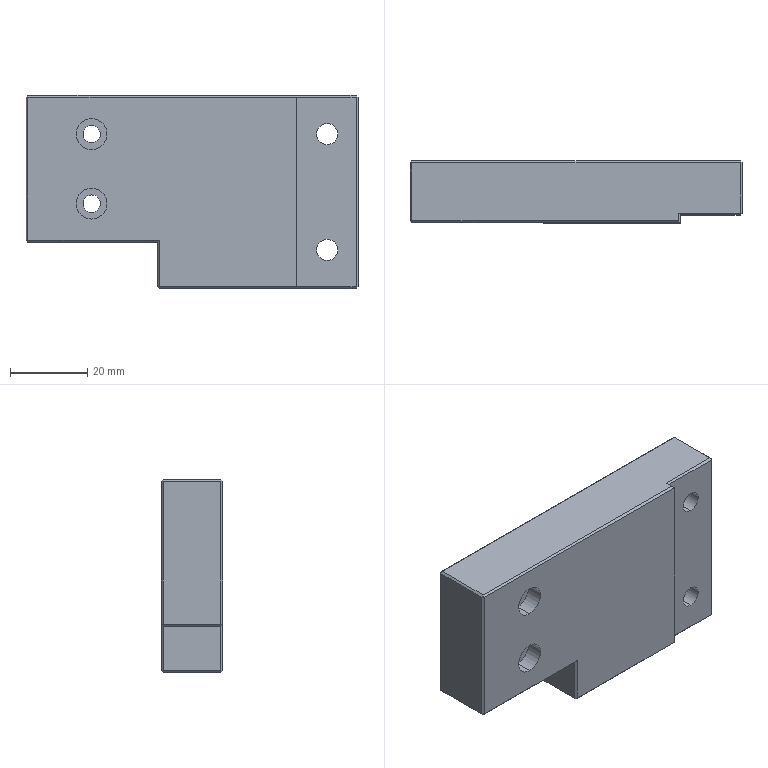Part | STEP file | ND25021-01-JDKM-57-TL | 1 solid | 69 faces | box 86 x 16 x 50 mm | volume 58348 mm3 | plane 45 | cylinder 20 | cone 4 | commonest cylinder face diameters 3.3 x4 4.5 x4 5.5 x4 8 x4 10 x4